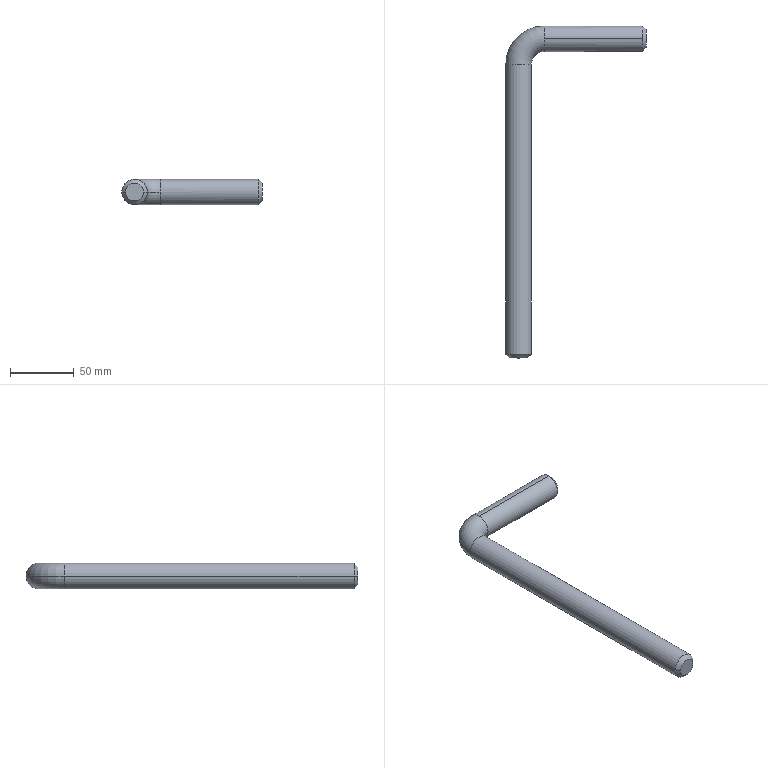Part | SolidWorks | features Chamfer 2, Sweep 1 | 1 solid | 12 faces | box 110 x 260 x 20 mm | volume 106750 mm3 | cone 4 | cylinder 4 | torus 2 | plane 2 | commonest cylinder face diameters 20 x4
STEP:
#1=CARTESIAN_POINT('',(-10.,-20.,0.));
#2=VERTEX_POINT('',#1);
#3=CARTESIAN_POINT('',(10.,-20.,0.));
#4=VERTEX_POINT('',#3);
#5=CARTESIAN_POINT('',(0.,-20.,0.));
#6=DIRECTION('',(0.,-1.,0.));
#7=DIRECTION('',(0.,0.,1.));
#8=AXIS2_PLACEMENT_3D('',#5,#6,#7);
#9=CIRCLE('',#8,10.);
#10=EDGE_CURVE('',#2,#4,#9,.T.);
#11=ORIENTED_EDGE('',*,*,#10,.F.);
#12=CARTESIAN_POINT('',(20.,10.,0.));
#13=VERTEX_POINT('',#12);
#14=CARTESIAN_POINT('',(20.,-20.,0.));
#15=DIRECTION('',(0.,0.,-1.));
#16=DIRECTION('',(-1.,0.,0.));
#17=AXIS2_PLACEMENT_3D('',#14,#15,#16);
#18=CIRCLE('',#17,30.);
#19=EDGE_CURVE('',#2,#13,#18,.T.);
#20=ORIENTED_EDGE('',*,*,#19,.T.);
#21=CARTESIAN_POINT('',(20.,0.,-10.));
#22=VERTEX_POINT('',#21);
#23=CARTESIAN_POINT('',(20.,0.,0.));
#24=DIRECTION('',(-1.,0.,0.));
#25=DIRECTION('',(0.,0.,1.));
#26=AXIS2_PLACEMENT_3D('',#23,#24,#25);
#27=CIRCLE('',#26,10.);
#28=EDGE_CURVE('',#13,#22,#27,.T.);
#29=ORIENTED_EDGE('',*,*,#28,.T.);
#30=CARTESIAN_POINT('',(20.,-10.,0.));
#31=VERTEX_POINT('',#30);
#32=CARTESIAN_POINT('',(20.,0.,0.));
#33=DIRECTION('',(-1.,0.,0.));
#34=DIRECTION('',(0.,0.,1.));
#35=AXIS2_PLACEMENT_3D('',#32,#33,#34);
#36=CIRCLE('',#35,10.);
#37=EDGE_CURVE('',#22,#31,#36,.T.);
#38=ORIENTED_EDGE('',*,*,#37,.T.);
#39=CARTESIAN_POINT('',(20.,-20.,0.));
#40=DIRECTION('',(0.,0.,-1.));
#41=DIRECTION('',(-1.,0.,0.));
#42=AXIS2_PLACEMENT_3D('',#39,#40,#41);
#43=CIRCLE('',#42,10.);
#44=EDGE_CURVE('',#4,#31,#43,.T.);
#45=ORIENTED_EDGE('',*,*,#44,.F.);
#46=EDGE_LOOP('',(#11,#20,#29,#38,#45));
#47=FACE_OUTER_BOUND('',#46,.T.);
#48=CARTESIAN_POINT('',(20.,-20.,0.));
#49=DIRECTION('',(0.,0.,-1.));
#50=DIRECTION('',(-1.,0.,0.));
#51=AXIS2_PLACEMENT_3D('',#48,#49,#50);
#52=TOROIDAL_SURFACE('',#51,20.,10.);
#53=ADVANCED_FACE('',(#47),#52,.T.);
#54=CARTESIAN_POINT('',(100.,0.,-7.));
#55=VERTEX_POINT('',#54);
#56=CARTESIAN_POINT('',(100.,0.,7.));
#57=VERTEX_POINT('',#56);
#58=CARTESIAN_POINT('',(100.,0.,0.));
#59=DIRECTION('',(1.,0.,0.));
#60=DIRECTION('',(0.,0.,1.));
#61=AXIS2_PLACEMENT_3D('',#58,#59,#60);
#62=CIRCLE('',#61,7.);
#63=EDGE_CURVE('',#55,#57,#62,.T.);
#64=ORIENTED_EDGE('',*,*,#63,.F.);
#65=CARTESIAN_POINT('',(97.,0.,-10.));
#66=VERTEX_POINT('',#65);
#67=CARTESIAN_POINT('',(97.,0.,-10.));
#68=DIRECTION('',(-0.7071,0.,-0.7071));
#69=VECTOR('',#68,1000.);
#70=LINE('',#67,#69);
#71=EDGE_CURVE('',#55,#66,#70,.T.);
#72=ORIENTED_EDGE('',*,*,#71,.T.);
#73=CARTESIAN_POINT('',(97.,0.,10.));
#74=VERTEX_POINT('',#73);
#75=CARTESIAN_POINT('',(97.,0.,0.));
#76=DIRECTION('',(-1.,0.,0.));
#77=DIRECTION('',(0.,0.,1.));
#78=AXIS2_PLACEMENT_3D('',#75,#76,#77);
#79=CIRCLE('',#78,10.);
#80=EDGE_CURVE('',#74,#66,#79,.T.);
#81=ORIENTED_EDGE('',*,*,#80,.F.);
#82=CARTESIAN_POINT('',(97.,0.,10.));
#83=DIRECTION('',(-0.7071,0.,0.7071));
#84=VECTOR('',#83,1000.);
#85=LINE('',#82,#84);
#86=EDGE_CURVE('',#57,#74,#85,.T.);
#87=ORIENTED_EDGE('',*,*,#86,.F.);
#88=EDGE_LOOP('',(#64,#72,#81,#87));
#89=FACE_OUTER_BOUND('',#88,.T.);
#90=CARTESIAN_POINT('',(97.,0.,0.));
#91=DIRECTION('',(-1.,0.,0.));
#92=DIRECTION('',(0.,0.,1.));
#93=AXIS2_PLACEMENT_3D('',#90,#91,#92);
#94=CONICAL_SURFACE('',#93,10.,0.7854);
#95=ADVANCED_FACE('',(#89),#94,.T.);
#96=CARTESIAN_POINT('',(7.,-250.,0.));
#97=VERTEX_POINT('',#96);
#98=CARTESIAN_POINT('',(-7.,-250.,0.));
#99=VERTEX_POINT('',#98);
#100=CARTESIAN_POINT('',(0.,-250.,0.));
#101=DIRECTION('',(0.,-1.,0.));
#102=DIRECTION('',(1.,0.,0.));
#103=AXIS2_PLACEMENT_3D('',#100,#101,#102);
#104=CIRCLE('',#103,7.);
#105=EDGE_CURVE('',#97,#99,#104,.T.);
#106=ORIENTED_EDGE('',*,*,#105,.F.);
#107=CARTESIAN_POINT('',(10.,-247.,0.));
#108=VERTEX_POINT('',#107);
#109=CARTESIAN_POINT('',(7.,-250.,0.));
#110=DIRECTION('',(0.7071,0.7071,0.));
#111=VECTOR('',#110,1000.);
#112=LINE('',#109,#111);
#113=EDGE_CURVE('',#97,#108,#112,.T.);
#114=ORIENTED_EDGE('',*,*,#113,.T.);
#115=CARTESIAN_POINT('',(-10.,-247.,0.));
#116=VERTEX_POINT('',#115);
#117=CARTESIAN_POINT('',(0.,-247.,0.));
#118=DIRECTION('',(0.,1.,0.));
#119=DIRECTION('',(1.,0.,0.));
#120=AXIS2_PLACEMENT_3D('',#117,#118,#119);
#121=CIRCLE('',#120,10.);
#122=EDGE_CURVE('',#116,#108,#121,.T.);
#123=ORIENTED_EDGE('',*,*,#122,.F.);
#124=CARTESIAN_POINT('',(-7.,-250.,0.));
#125=DIRECTION('',(-0.7071,0.7071,0.));
#126=VECTOR('',#125,1000.);
#127=LINE('',#124,#126);
#128=EDGE_CURVE('',#99,#116,#127,.T.);
#129=ORIENTED_EDGE('',*,*,#128,.F.);
#130=EDGE_LOOP('',(#106,#114,#123,#129));
#131=FACE_OUTER_BOUND('',#130,.T.);
#132=CARTESIAN_POINT('',(0.,-250.,0.));
#133=DIRECTION('',(0.,1.,0.));
#134=DIRECTION('',(-1.,0.,0.));
#135=AXIS2_PLACEMENT_3D('',#132,#133,#134);
#136=CONICAL_SURFACE('',#135,7.,0.7854);
#137=ADVANCED_FACE('',(#131),#136,.T.);
#138=CARTESIAN_POINT('',(20.,0.,10.));
#139=VERTEX_POINT('',#138);
#140=CARTESIAN_POINT('',(20.,0.,0.));
#141=DIRECTION('',(-1.,0.,0.));
#142=DIRECTION('',(0.,0.,1.));
#143=AXIS2_PLACEMENT_3D('',#140,#141,#142);
#144=CIRCLE('',#143,10.);
#145=EDGE_CURVE('',#139,#13,#144,.T.);
#146=ORIENTED_EDGE('',*,*,#145,.F.);
#147=CARTESIAN_POINT('',(20.,0.,10.));
#148=DIRECTION('',(1.,0.,0.));
#149=VECTOR('',#148,1000.);
#150=LINE('',#147,#149);
#151=EDGE_CURVE('',#139,#74,#150,.T.);
#152=ORIENTED_EDGE('',*,*,#151,.T.);
#153=ORIENTED_EDGE('',*,*,#80,.T.);
#154=CARTESIAN_POINT('',(20.,0.,-10.));
#155=DIRECTION('',(1.,0.,0.));
#156=VECTOR('',#155,1000.);
#157=LINE('',#154,#156);
#158=EDGE_CURVE('',#22,#66,#157,.T.);
#159=ORIENTED_EDGE('',*,*,#158,.F.);
#160=ORIENTED_EDGE('',*,*,#28,.F.);
#161=EDGE_LOOP('',(#146,#152,#153,#159,#160));
#162=FACE_OUTER_BOUND('',#161,.T.);
#163=CARTESIAN_POINT('',(20.,0.,0.));
#164=DIRECTION('',(1.,0.,0.));
#165=DIRECTION('',(0.,0.,-1.));
#166=AXIS2_PLACEMENT_3D('',#163,#164,#165);
#167=CYLINDRICAL_SURFACE('',#166,10.);
#168=ADVANCED_FACE('',(#162),#167,.T.);
#169=ORIENTED_EDGE('',*,*,#122,.T.);
#170=CARTESIAN_POINT('',(10.,-250.,0.));
#171=DIRECTION('',(0.,1.,0.));
#172=VECTOR('',#171,1000.);
#173=LINE('',#170,#172);
#174=EDGE_CURVE('',#108,#4,#173,.T.);
#175=ORIENTED_EDGE('',*,*,#174,.T.);
#176=CARTESIAN_POINT('',(0.,-20.,0.));
#177=DIRECTION('',(0.,-1.,0.));
#178=DIRECTION('',(0.,0.,1.));
#179=AXIS2_PLACEMENT_3D('',#176,#177,#178);
#180=CIRCLE('',#179,10.);
#181=EDGE_CURVE('',#4,#2,#180,.T.);
#182=ORIENTED_EDGE('',*,*,#181,.T.);
#183=CARTESIAN_POINT('',(-10.,-250.,0.));
#184=DIRECTION('',(0.,1.,0.));
#185=VECTOR('',#184,1000.);
#186=LINE('',#183,#185);
#187=EDGE_CURVE('',#116,#2,#186,.T.);
#188=ORIENTED_EDGE('',*,*,#187,.F.);
#189=EDGE_LOOP('',(#169,#175,#182,#188));
#190=FACE_OUTER_BOUND('',#189,.T.);
#191=CARTESIAN_POINT('',(0.,-250.,0.));
#192=DIRECTION('',(0.,1.,0.));
#193=DIRECTION('',(-1.,0.,0.));
#194=AXIS2_PLACEMENT_3D('',#191,#192,#193);
#195=CYLINDRICAL_SURFACE('',#194,10.);
#196=ADVANCED_FACE('',(#190),#195,.T.);
#197=ORIENTED_EDGE('',*,*,#151,.F.);
#198=CARTESIAN_POINT('',(20.,0.,0.));
#199=DIRECTION('',(-1.,0.,0.));
#200=DIRECTION('',(0.,0.,1.));
#201=AXIS2_PLACEMENT_3D('',#198,#199,#200);
#202=CIRCLE('',#201,10.);
#203=EDGE_CURVE('',#31,#139,#202,.T.);
#204=ORIENTED_EDGE('',*,*,#203,.F.);
#205=ORIENTED_EDGE('',*,*,#37,.F.);
#206=ORIENTED_EDGE('',*,*,#158,.T.);
#207=CARTESIAN_POINT('',(97.,0.,0.));
#208=DIRECTION('',(-1.,0.,0.));
#209=DIRECTION('',(0.,0.,1.));
#210=AXIS2_PLACEMENT_3D('',#207,#208,#209);
#211=CIRCLE('',#210,10.);
#212=EDGE_CURVE('',#66,#74,#211,.T.);
#213=ORIENTED_EDGE('',*,*,#212,.T.);
#214=EDGE_LOOP('',(#197,#204,#205,#206,#213));
#215=FACE_OUTER_BOUND('',#214,.T.);
#216=CARTESIAN_POINT('',(20.,0.,0.));
#217=DIRECTION('',(1.,0.,0.));
#218=DIRECTION('',(0.,0.,-1.));
#219=AXIS2_PLACEMENT_3D('',#216,#217,#218);
#220=CYLINDRICAL_SURFACE('',#219,10.);
#221=ADVANCED_FACE('',(#215),#220,.T.);
#222=ORIENTED_EDGE('',*,*,#19,.F.);
#223=ORIENTED_EDGE('',*,*,#181,.F.);
#224=ORIENTED_EDGE('',*,*,#44,.T.);
#225=ORIENTED_EDGE('',*,*,#203,.T.);
#226=ORIENTED_EDGE('',*,*,#145,.T.);
#227=EDGE_LOOP('',(#222,#223,#224,#225,#226));
#228=FACE_OUTER_BOUND('',#227,.T.);
#229=CARTESIAN_POINT('',(20.,-20.,0.));
#230=DIRECTION('',(0.,0.,-1.));
#231=DIRECTION('',(-1.,0.,0.));
#232=AXIS2_PLACEMENT_3D('',#229,#230,#231);
#233=TOROIDAL_SURFACE('',#232,20.,10.);
#234=ADVANCED_FACE('',(#228),#233,.T.);
#235=ORIENTED_EDGE('',*,*,#174,.F.);
#236=CARTESIAN_POINT('',(0.,-247.,0.));
#237=DIRECTION('',(0.,1.,0.));
#238=DIRECTION('',(1.,0.,0.));
#239=AXIS2_PLACEMENT_3D('',#236,#237,#238);
#240=CIRCLE('',#239,10.);
#241=EDGE_CURVE('',#108,#116,#240,.T.);
#242=ORIENTED_EDGE('',*,*,#241,.T.);
#243=ORIENTED_EDGE('',*,*,#187,.T.);
#244=ORIENTED_EDGE('',*,*,#10,.T.);
#245=EDGE_LOOP('',(#235,#242,#243,#244));
#246=FACE_OUTER_BOUND('',#245,.T.);
#247=CARTESIAN_POINT('',(0.,-250.,0.));
#248=DIRECTION('',(0.,1.,0.));
#249=DIRECTION('',(-1.,0.,0.));
#250=AXIS2_PLACEMENT_3D('',#247,#248,#249);
#251=CYLINDRICAL_SURFACE('',#250,10.);
#252=ADVANCED_FACE('',(#246),#251,.T.);
#253=CARTESIAN_POINT('',(100.,0.,0.));
#254=DIRECTION('',(1.,0.,0.));
#255=DIRECTION('',(0.,0.,1.));
#256=AXIS2_PLACEMENT_3D('',#253,#254,#255);
#257=CIRCLE('',#256,7.);
#258=EDGE_CURVE('',#57,#55,#257,.T.);
#259=ORIENTED_EDGE('',*,*,#258,.T.);
#260=ORIENTED_EDGE('',*,*,#63,.T.);
#261=EDGE_LOOP('',(#259,#260));
#262=FACE_OUTER_BOUND('',#261,.T.);
#263=CARTESIAN_POINT('',(100.,0.,0.));
#264=DIRECTION('',(-1.,0.,0.));
#265=DIRECTION('',(0.,0.,1.));
#266=AXIS2_PLACEMENT_3D('',#263,#264,#265);
#267=PLANE('',#266);
#268=ADVANCED_FACE('',(#262),#267,.F.);
#269=CARTESIAN_POINT('',(0.,-250.,0.));
#270=DIRECTION('',(0.,-1.,0.));
#271=DIRECTION('',(1.,0.,0.));
#272=AXIS2_PLACEMENT_3D('',#269,#270,#271);
#273=CIRCLE('',#272,7.);
#274=EDGE_CURVE('',#99,#97,#273,.T.);
#275=ORIENTED_EDGE('',*,*,#274,.T.);
#276=ORIENTED_EDGE('',*,*,#105,.T.);
#277=EDGE_LOOP('',(#275,#276));
#278=FACE_OUTER_BOUND('',#277,.T.);
#279=CARTESIAN_POINT('',(0.,-250.,0.));
#280=DIRECTION('',(0.,-1.,0.));
#281=DIRECTION('',(0.,0.,1.));
#282=AXIS2_PLACEMENT_3D('',#279,#280,#281);
#283=PLANE('',#282);
#284=ADVANCED_FACE('',(#278),#283,.T.);
#285=ORIENTED_EDGE('',*,*,#113,.F.);
#286=ORIENTED_EDGE('',*,*,#274,.F.);
#287=ORIENTED_EDGE('',*,*,#128,.T.);
#288=ORIENTED_EDGE('',*,*,#241,.F.);
#289=EDGE_LOOP('',(#285,#286,#287,#288));
#290=FACE_OUTER_BOUND('',#289,.T.);
#291=CARTESIAN_POINT('',(0.,-250.,0.));
#292=DIRECTION('',(0.,1.,0.));
#293=DIRECTION('',(-1.,0.,0.));
#294=AXIS2_PLACEMENT_3D('',#291,#292,#293);
#295=CONICAL_SURFACE('',#294,7.,0.7854);
#296=ADVANCED_FACE('',(#290),#295,.T.);
#297=ORIENTED_EDGE('',*,*,#71,.F.);
#298=ORIENTED_EDGE('',*,*,#258,.F.);
#299=ORIENTED_EDGE('',*,*,#86,.T.);
#300=ORIENTED_EDGE('',*,*,#212,.F.);
#301=EDGE_LOOP('',(#297,#298,#299,#300));
#302=FACE_OUTER_BOUND('',#301,.T.);
#303=CARTESIAN_POINT('',(97.,0.,0.));
#304=DIRECTION('',(-1.,0.,0.));
#305=DIRECTION('',(0.,0.,1.));
#306=AXIS2_PLACEMENT_3D('',#303,#304,#305);
#307=CONICAL_SURFACE('',#306,10.,0.7854);
#308=ADVANCED_FACE('',(#302),#307,.T.);
#309=CLOSED_SHELL('',(#53,#95,#137,#168,#196,#221,#234,#252,#268,#284,#296,#308));
#310=MANIFOLD_SOLID_BREP('',#309);
#311=CARTESIAN_POINT('',(0.,0.,0.));
#312=DIRECTION('',(0.,0.,1.));
#313=DIRECTION('',(1.,0.,0.));
#314=AXIS2_PLACEMENT_3D('',#311,#312,#313);
#315=(LENGTH_UNIT()NAMED_UNIT(*)SI_UNIT(.MILLI.,.METRE.));
#316=UNCERTAINTY_MEASURE_WITH_UNIT(LENGTH_MEASURE(0.00001),#315,'','');
#317=(NAMED_UNIT(*)PLANE_ANGLE_UNIT()SI_UNIT($,.RADIAN.));
#318=(NAMED_UNIT(*)SI_UNIT($,.STERADIAN.)SOLID_ANGLE_UNIT());
#319=(GEOMETRIC_REPRESENTATION_CONTEXT(3)GLOBAL_UNCERTAINTY_ASSIGNED_CONTEXT((#316))GLOBAL_UNIT_ASSIGNED_CONTEXT((#315,#317,#318))REPRESENTATION_CONTEXT('',''));
#320=ADVANCED_BREP_SHAPE_REPRESENTATION('',(#310,#314),#319);